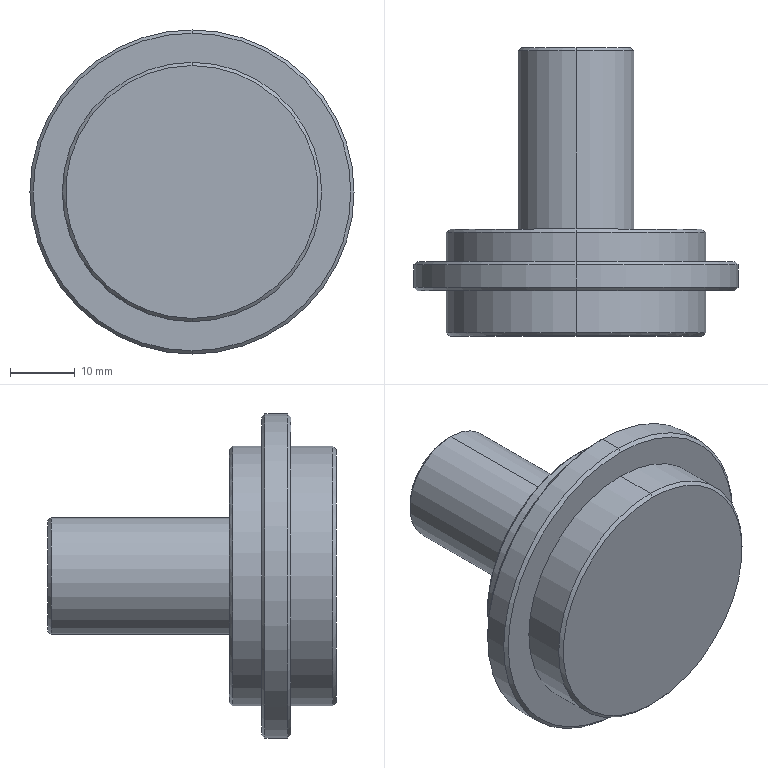Part | SolidWorks | features Chamfer 1, Revolution 1 | 1 solid | 23 faces | box 50 x 44.5 x 50 mm | volume 30963 mm3 | cone 10 | cylinder 8 | plane 5 | commonest cylinder face diameters 40 x4 18 x2 50 x2
STEP:
#1=CARTESIAN_POINT('',(249.314,-567.,8.5));
#2=VERTEX_POINT('',#1);
#3=CARTESIAN_POINT('',(249.314,-567.,-8.5));
#4=VERTEX_POINT('',#3);
#5=CARTESIAN_POINT('',(249.314,-567.,0.));
#6=DIRECTION('',(0.,1.,0.));
#7=DIRECTION('',(0.,0.,-1.));
#8=AXIS2_PLACEMENT_3D('',#5,#6,#7);
#9=CIRCLE('',#8,8.5);
#10=EDGE_CURVE('',#2,#4,#9,.T.);
#11=ORIENTED_EDGE('',*,*,#10,.F.);
#12=CARTESIAN_POINT('',(249.314,-567.5,9.));
#13=VERTEX_POINT('',#12);
#14=CARTESIAN_POINT('',(249.314,-567.,8.5));
#15=DIRECTION('',(0.,-0.7071,0.7071));
#16=VECTOR('',#15,1000.);
#17=LINE('',#14,#16);
#18=EDGE_CURVE('',#2,#13,#17,.T.);
#19=ORIENTED_EDGE('',*,*,#18,.T.);
#20=CARTESIAN_POINT('',(249.314,-567.5,-9.));
#21=VERTEX_POINT('',#20);
#22=CARTESIAN_POINT('',(249.314,-567.5,0.));
#23=DIRECTION('',(0.,-1.,0.));
#24=DIRECTION('',(0.,0.,-1.));
#25=AXIS2_PLACEMENT_3D('',#22,#23,#24);
#26=CIRCLE('',#25,9.);
#27=EDGE_CURVE('',#21,#13,#26,.T.);
#28=ORIENTED_EDGE('',*,*,#27,.F.);
#29=CARTESIAN_POINT('',(249.314,-567.,-8.5));
#30=DIRECTION('',(0.,-0.7071,-0.7071));
#31=VECTOR('',#30,1000.);
#32=LINE('',#29,#31);
#33=EDGE_CURVE('',#4,#21,#32,.T.);
#34=ORIENTED_EDGE('',*,*,#33,.F.);
#35=EDGE_LOOP('',(#11,#19,#28,#34));
#36=FACE_OUTER_BOUND('',#35,.T.);
#37=CARTESIAN_POINT('',(249.314,-567.,0.));
#38=DIRECTION('',(0.,-1.,0.));
#39=DIRECTION('',(0.,0.,-1.));
#40=AXIS2_PLACEMENT_3D('',#37,#38,#39);
#41=CONICAL_SURFACE('',#40,8.5,0.7854);
#42=ADVANCED_FACE('',(#36),#41,.T.);
#43=CARTESIAN_POINT('',(249.314,-595.,19.5));
#44=VERTEX_POINT('',#43);
#45=CARTESIAN_POINT('',(249.314,-595.,-19.5));
#46=VERTEX_POINT('',#45);
#47=CARTESIAN_POINT('',(249.314,-595.,0.));
#48=DIRECTION('',(0.,1.,0.));
#49=DIRECTION('',(0.,0.,-1.));
#50=AXIS2_PLACEMENT_3D('',#47,#48,#49);
#51=CIRCLE('',#50,19.5);
#52=EDGE_CURVE('',#44,#46,#51,.T.);
#53=ORIENTED_EDGE('',*,*,#52,.F.);
#54=CARTESIAN_POINT('',(249.314,-595.5,20.));
#55=VERTEX_POINT('',#54);
#56=CARTESIAN_POINT('',(249.314,-595.,19.5));
#57=DIRECTION('',(0.,-0.7071,0.7071));
#58=VECTOR('',#57,1000.);
#59=LINE('',#56,#58);
#60=EDGE_CURVE('',#44,#55,#59,.T.);
#61=ORIENTED_EDGE('',*,*,#60,.T.);
#62=CARTESIAN_POINT('',(249.314,-595.5,-20.));
#63=VERTEX_POINT('',#62);
#64=CARTESIAN_POINT('',(249.314,-595.5,0.));
#65=DIRECTION('',(0.,-1.,0.));
#66=DIRECTION('',(0.,0.,-1.));
#67=AXIS2_PLACEMENT_3D('',#64,#65,#66);
#68=CIRCLE('',#67,20.);
#69=EDGE_CURVE('',#63,#55,#68,.T.);
#70=ORIENTED_EDGE('',*,*,#69,.F.);
#71=CARTESIAN_POINT('',(249.314,-595.,-19.5));
#72=DIRECTION('',(0.,-0.7071,-0.7071));
#73=VECTOR('',#72,1000.);
#74=LINE('',#71,#73);
#75=EDGE_CURVE('',#46,#63,#74,.T.);
#76=ORIENTED_EDGE('',*,*,#75,.F.);
#77=EDGE_LOOP('',(#53,#61,#70,#76));
#78=FACE_OUTER_BOUND('',#77,.T.);
#79=CARTESIAN_POINT('',(249.314,-595.,0.));
#80=DIRECTION('',(0.,-1.,0.));
#81=DIRECTION('',(0.,0.,-1.));
#82=AXIS2_PLACEMENT_3D('',#79,#80,#81);
#83=CONICAL_SURFACE('',#82,19.5,0.7854);
#84=ADVANCED_FACE('',(#78),#83,.T.);
#85=CARTESIAN_POINT('',(249.314,-600.,24.5));
#86=VERTEX_POINT('',#85);
#87=CARTESIAN_POINT('',(249.314,-600.,-24.5));
#88=VERTEX_POINT('',#87);
#89=CARTESIAN_POINT('',(249.314,-600.,0.));
#90=DIRECTION('',(0.,1.,0.));
#91=DIRECTION('',(0.,0.,-1.));
#92=AXIS2_PLACEMENT_3D('',#89,#90,#91);
#93=CIRCLE('',#92,24.5);
#94=EDGE_CURVE('',#86,#88,#93,.T.);
#95=ORIENTED_EDGE('',*,*,#94,.F.);
#96=CARTESIAN_POINT('',(249.314,-600.5,25.));
#97=VERTEX_POINT('',#96);
#98=CARTESIAN_POINT('',(249.314,-600.,24.5));
#99=DIRECTION('',(0.,-0.7071,0.7071));
#100=VECTOR('',#99,1000.);
#101=LINE('',#98,#100);
#102=EDGE_CURVE('',#86,#97,#101,.T.);
#103=ORIENTED_EDGE('',*,*,#102,.T.);
#104=CARTESIAN_POINT('',(249.314,-600.5,-25.));
#105=VERTEX_POINT('',#104);
#106=CARTESIAN_POINT('',(249.314,-600.5,0.));
#107=DIRECTION('',(0.,-1.,0.));
#108=DIRECTION('',(0.,0.,-1.));
#109=AXIS2_PLACEMENT_3D('',#106,#107,#108);
#110=CIRCLE('',#109,25.);
#111=EDGE_CURVE('',#105,#97,#110,.T.);
#112=ORIENTED_EDGE('',*,*,#111,.F.);
#113=CARTESIAN_POINT('',(249.314,-600.,-24.5));
#114=DIRECTION('',(0.,-0.7071,-0.7071));
#115=VECTOR('',#114,1000.);
#116=LINE('',#113,#115);
#117=EDGE_CURVE('',#88,#105,#116,.T.);
#118=ORIENTED_EDGE('',*,*,#117,.F.);
#119=EDGE_LOOP('',(#95,#103,#112,#118));
#120=FACE_OUTER_BOUND('',#119,.T.);
#121=CARTESIAN_POINT('',(249.314,-600.,0.));
#122=DIRECTION('',(0.,-1.,0.));
#123=DIRECTION('',(0.,0.,-1.));
#124=AXIS2_PLACEMENT_3D('',#121,#122,#123);
#125=CONICAL_SURFACE('',#124,24.5,0.7854);
#126=ADVANCED_FACE('',(#120),#125,.T.);
#127=CARTESIAN_POINT('',(249.314,-604.5,-24.5));
#128=VERTEX_POINT('',#127);
#129=CARTESIAN_POINT('',(249.314,-604.5,24.5));
#130=VERTEX_POINT('',#129);
#131=CARTESIAN_POINT('',(249.314,-604.5,0.));
#132=DIRECTION('',(0.,-1.,0.));
#133=DIRECTION('',(0.,0.,1.));
#134=AXIS2_PLACEMENT_3D('',#131,#132,#133);
#135=CIRCLE('',#134,24.5);
#136=EDGE_CURVE('',#128,#130,#135,.T.);
#137=ORIENTED_EDGE('',*,*,#136,.F.);
#138=CARTESIAN_POINT('',(249.314,-604.,-25.));
#139=VERTEX_POINT('',#138);
#140=CARTESIAN_POINT('',(249.314,-604.,-25.));
#141=DIRECTION('',(0.,0.7071,-0.7071));
#142=VECTOR('',#141,1000.);
#143=LINE('',#140,#142);
#144=EDGE_CURVE('',#128,#139,#143,.T.);
#145=ORIENTED_EDGE('',*,*,#144,.T.);
#146=CARTESIAN_POINT('',(249.314,-604.,25.));
#147=VERTEX_POINT('',#146);
#148=CARTESIAN_POINT('',(249.314,-604.,0.));
#149=DIRECTION('',(0.,1.,0.));
#150=DIRECTION('',(0.,0.,1.));
#151=AXIS2_PLACEMENT_3D('',#148,#149,#150);
#152=CIRCLE('',#151,25.);
#153=EDGE_CURVE('',#147,#139,#152,.T.);
#154=ORIENTED_EDGE('',*,*,#153,.F.);
#155=CARTESIAN_POINT('',(249.314,-604.,25.));
#156=DIRECTION('',(0.,0.7071,0.7071));
#157=VECTOR('',#156,1000.);
#158=LINE('',#155,#157);
#159=EDGE_CURVE('',#130,#147,#158,.T.);
#160=ORIENTED_EDGE('',*,*,#159,.F.);
#161=EDGE_LOOP('',(#137,#145,#154,#160));
#162=FACE_OUTER_BOUND('',#161,.T.);
#163=CARTESIAN_POINT('',(249.314,-604.,0.));
#164=DIRECTION('',(0.,1.,0.));
#165=DIRECTION('',(0.,0.,1.));
#166=AXIS2_PLACEMENT_3D('',#163,#164,#165);
#167=CONICAL_SURFACE('',#166,25.,0.7854);
#168=ADVANCED_FACE('',(#162),#167,.T.);
#169=CARTESIAN_POINT('',(249.314,-611.5,-19.5));
#170=VERTEX_POINT('',#169);
#171=CARTESIAN_POINT('',(249.314,-611.5,19.5));
#172=VERTEX_POINT('',#171);
#173=CARTESIAN_POINT('',(249.314,-611.5,0.));
#174=DIRECTION('',(0.,-1.,0.));
#175=DIRECTION('',(0.,0.,1.));
#176=AXIS2_PLACEMENT_3D('',#173,#174,#175);
#177=CIRCLE('',#176,19.5);
#178=EDGE_CURVE('',#170,#172,#177,.T.);
#179=ORIENTED_EDGE('',*,*,#178,.F.);
#180=CARTESIAN_POINT('',(249.314,-611.,-20.));
#181=VERTEX_POINT('',#180);
#182=CARTESIAN_POINT('',(249.314,-611.,-20.));
#183=DIRECTION('',(0.,0.7071,-0.7071));
#184=VECTOR('',#183,1000.);
#185=LINE('',#182,#184);
#186=EDGE_CURVE('',#170,#181,#185,.T.);
#187=ORIENTED_EDGE('',*,*,#186,.T.);
#188=CARTESIAN_POINT('',(249.314,-611.,20.));
#189=VERTEX_POINT('',#188);
#190=CARTESIAN_POINT('',(249.314,-611.,0.));
#191=DIRECTION('',(0.,1.,0.));
#192=DIRECTION('',(0.,0.,1.));
#193=AXIS2_PLACEMENT_3D('',#190,#191,#192);
#194=CIRCLE('',#193,20.);
#195=EDGE_CURVE('',#189,#181,#194,.T.);
#196=ORIENTED_EDGE('',*,*,#195,.F.);
#197=CARTESIAN_POINT('',(249.314,-611.,20.));
#198=DIRECTION('',(0.,0.7071,0.7071));
#199=VECTOR('',#198,1000.);
#200=LINE('',#197,#199);
#201=EDGE_CURVE('',#172,#189,#200,.T.);
#202=ORIENTED_EDGE('',*,*,#201,.F.);
#203=EDGE_LOOP('',(#179,#187,#196,#202));
#204=FACE_OUTER_BOUND('',#203,.T.);
#205=CARTESIAN_POINT('',(249.314,-611.,0.));
#206=DIRECTION('',(0.,1.,0.));
#207=DIRECTION('',(0.,0.,1.));
#208=AXIS2_PLACEMENT_3D('',#205,#206,#207);
#209=CONICAL_SURFACE('',#208,20.,0.7854);
#210=ADVANCED_FACE('',(#204),#209,.T.);
#211=CARTESIAN_POINT('',(249.314,-595.,9.));
#212=VERTEX_POINT('',#211);
#213=CARTESIAN_POINT('',(249.314,-595.,-9.));
#214=VERTEX_POINT('',#213);
#215=CARTESIAN_POINT('',(249.314,-595.,0.));
#216=DIRECTION('',(0.,1.,0.));
#217=DIRECTION('',(0.,0.,1.));
#218=AXIS2_PLACEMENT_3D('',#215,#216,#217);
#219=CIRCLE('',#218,9.);
#220=EDGE_CURVE('',#212,#214,#219,.T.);
#221=ORIENTED_EDGE('',*,*,#220,.T.);
#222=CARTESIAN_POINT('',(249.314,-567.,-9.));
#223=DIRECTION('',(0.,1.,0.));
#224=VECTOR('',#223,1000.);
#225=LINE('',#222,#224);
#226=EDGE_CURVE('',#214,#21,#225,.T.);
#227=ORIENTED_EDGE('',*,*,#226,.T.);
#228=ORIENTED_EDGE('',*,*,#27,.T.);
#229=CARTESIAN_POINT('',(249.314,-567.,9.));
#230=DIRECTION('',(0.,1.,0.));
#231=VECTOR('',#230,1000.);
#232=LINE('',#229,#231);
#233=EDGE_CURVE('',#212,#13,#232,.T.);
#234=ORIENTED_EDGE('',*,*,#233,.F.);
#235=EDGE_LOOP('',(#221,#227,#228,#234));
#236=FACE_OUTER_BOUND('',#235,.T.);
#237=CARTESIAN_POINT('',(249.314,-567.,0.));
#238=DIRECTION('',(0.,1.,0.));
#239=DIRECTION('',(0.,0.,1.));
#240=AXIS2_PLACEMENT_3D('',#237,#238,#239);
#241=CYLINDRICAL_SURFACE('',#240,9.);
#242=ADVANCED_FACE('',(#236),#241,.T.);
#243=CARTESIAN_POINT('',(249.314,-600.,20.));
#244=VERTEX_POINT('',#243);
#245=CARTESIAN_POINT('',(249.314,-600.,-20.));
#246=VERTEX_POINT('',#245);
#247=CARTESIAN_POINT('',(249.314,-600.,0.));
#248=DIRECTION('',(0.,1.,0.));
#249=DIRECTION('',(0.,0.,1.));
#250=AXIS2_PLACEMENT_3D('',#247,#248,#249);
#251=CIRCLE('',#250,20.);
#252=EDGE_CURVE('',#244,#246,#251,.T.);
#253=ORIENTED_EDGE('',*,*,#252,.T.);
#254=CARTESIAN_POINT('',(249.314,-567.,-20.));
#255=DIRECTION('',(0.,1.,0.));
#256=VECTOR('',#255,1000.);
#257=LINE('',#254,#256);
#258=EDGE_CURVE('',#246,#63,#257,.T.);
#259=ORIENTED_EDGE('',*,*,#258,.T.);
#260=ORIENTED_EDGE('',*,*,#69,.T.);
#261=CARTESIAN_POINT('',(249.314,-567.,20.));
#262=DIRECTION('',(0.,1.,0.));
#263=VECTOR('',#262,1000.);
#264=LINE('',#261,#263);
#265=EDGE_CURVE('',#244,#55,#264,.T.);
#266=ORIENTED_EDGE('',*,*,#265,.F.);
#267=EDGE_LOOP('',(#253,#259,#260,#266));
#268=FACE_OUTER_BOUND('',#267,.T.);
#269=CARTESIAN_POINT('',(249.314,-567.,0.));
#270=DIRECTION('',(0.,1.,0.));
#271=DIRECTION('',(0.,0.,1.));
#272=AXIS2_PLACEMENT_3D('',#269,#270,#271);
#273=CYLINDRICAL_SURFACE('',#272,20.);
#274=ADVANCED_FACE('',(#268),#273,.T.);
#275=ORIENTED_EDGE('',*,*,#153,.T.);
#276=CARTESIAN_POINT('',(249.314,-567.,-25.));
#277=DIRECTION('',(0.,1.,0.));
#278=VECTOR('',#277,1000.);
#279=LINE('',#276,#278);
#280=EDGE_CURVE('',#139,#105,#279,.T.);
#281=ORIENTED_EDGE('',*,*,#280,.T.);
#282=ORIENTED_EDGE('',*,*,#111,.T.);
#283=CARTESIAN_POINT('',(249.314,-567.,25.));
#284=DIRECTION('',(0.,1.,0.));
#285=VECTOR('',#284,1000.);
#286=LINE('',#283,#285);
#287=EDGE_CURVE('',#147,#97,#286,.T.);
#288=ORIENTED_EDGE('',*,*,#287,.F.);
#289=EDGE_LOOP('',(#275,#281,#282,#288));
#290=FACE_OUTER_BOUND('',#289,.T.);
#291=CARTESIAN_POINT('',(249.314,-567.,0.));
#292=DIRECTION('',(0.,1.,0.));
#293=DIRECTION('',(0.,0.,1.));
#294=AXIS2_PLACEMENT_3D('',#291,#292,#293);
#295=CYLINDRICAL_SURFACE('',#294,25.);
#296=ADVANCED_FACE('',(#290),#295,.T.);
#297=ORIENTED_EDGE('',*,*,#195,.T.);
#298=CARTESIAN_POINT('',(249.314,-604.5,-20.));
#299=VERTEX_POINT('',#298);
#300=CARTESIAN_POINT('',(249.314,-567.,-20.));
#301=DIRECTION('',(0.,1.,0.));
#302=VECTOR('',#301,1000.);
#303=LINE('',#300,#302);
#304=EDGE_CURVE('',#181,#299,#303,.T.);
#305=ORIENTED_EDGE('',*,*,#304,.T.);
#306=CARTESIAN_POINT('',(249.314,-604.5,20.));
#307=VERTEX_POINT('',#306);
#308=CARTESIAN_POINT('',(249.314,-604.5,0.));
#309=DIRECTION('',(0.,1.,0.));
#310=DIRECTION('',(0.,0.,1.));
#311=AXIS2_PLACEMENT_3D('',#308,#309,#310);
#312=CIRCLE('',#311,20.);
#313=EDGE_CURVE('',#307,#299,#312,.T.);
#314=ORIENTED_EDGE('',*,*,#313,.F.);
#315=CARTESIAN_POINT('',(249.314,-567.,20.));
#316=DIRECTION('',(0.,1.,0.));
#317=VECTOR('',#316,1000.);
#318=LINE('',#315,#317);
#319=EDGE_CURVE('',#189,#307,#318,.T.);
#320=ORIENTED_EDGE('',*,*,#319,.F.);
#321=EDGE_LOOP('',(#297,#305,#314,#320));
#322=FACE_OUTER_BOUND('',#321,.T.);
#323=CARTESIAN_POINT('',(249.314,-567.,0.));
#324=DIRECTION('',(0.,1.,0.));
#325=DIRECTION('',(0.,0.,1.));
#326=AXIS2_PLACEMENT_3D('',#323,#324,#325);
#327=CYLINDRICAL_SURFACE('',#326,20.);
#328=ADVANCED_FACE('',(#322),#327,.T.);
#329=CARTESIAN_POINT('',(249.314,-567.,0.));
#330=DIRECTION('',(0.,1.,0.));
#331=DIRECTION('',(0.,0.,-1.));
#332=AXIS2_PLACEMENT_3D('',#329,#330,#331);
#333=CIRCLE('',#332,8.5);
#334=EDGE_CURVE('',#4,#2,#333,.T.);
#335=ORIENTED_EDGE('',*,*,#334,.T.);
#336=ORIENTED_EDGE('',*,*,#10,.T.);
#337=EDGE_LOOP('',(#335,#336));
#338=FACE_OUTER_BOUND('',#337,.T.);
#339=CARTESIAN_POINT('',(258.314,-567.,0.));
#340=DIRECTION('',(0.,-1.,0.));
#341=DIRECTION('',(0.,0.,-1.));
#342=AXIS2_PLACEMENT_3D('',#339,#340,#341);
#343=PLANE('',#342);
#344=ADVANCED_FACE('',(#338),#343,.F.);
#345=CARTESIAN_POINT('',(249.314,-611.5,0.));
#346=DIRECTION('',(0.,-1.,0.));
#347=DIRECTION('',(0.,0.,1.));
#348=AXIS2_PLACEMENT_3D('',#345,#346,#347);
#349=CIRCLE('',#348,19.5);
#350=EDGE_CURVE('',#172,#170,#349,.T.);
#351=ORIENTED_EDGE('',*,*,#350,.T.);
#352=ORIENTED_EDGE('',*,*,#178,.T.);
#353=EDGE_LOOP('',(#351,#352));
#354=FACE_OUTER_BOUND('',#353,.T.);
#355=CARTESIAN_POINT('',(269.314,-611.5,0.));
#356=DIRECTION('',(0.,1.,0.));
#357=DIRECTION('',(0.,0.,1.));
#358=AXIS2_PLACEMENT_3D('',#355,#356,#357);
#359=PLANE('',#358);
#360=ADVANCED_FACE('',(#354),#359,.F.);
#361=ORIENTED_EDGE('',*,*,#304,.F.);
#362=CARTESIAN_POINT('',(249.314,-611.,0.));
#363=DIRECTION('',(0.,1.,0.));
#364=DIRECTION('',(0.,0.,1.));
#365=AXIS2_PLACEMENT_3D('',#362,#363,#364);
#366=CIRCLE('',#365,20.);
#367=EDGE_CURVE('',#181,#189,#366,.T.);
#368=ORIENTED_EDGE('',*,*,#367,.T.);
#369=ORIENTED_EDGE('',*,*,#319,.T.);
#370=CARTESIAN_POINT('',(249.314,-604.5,0.));
#371=DIRECTION('',(0.,1.,0.));
#372=DIRECTION('',(0.,0.,1.));
#373=AXIS2_PLACEMENT_3D('',#370,#371,#372);
#374=CIRCLE('',#373,20.);
#375=EDGE_CURVE('',#299,#307,#374,.T.);
#376=ORIENTED_EDGE('',*,*,#375,.F.);
#377=EDGE_LOOP('',(#361,#368,#369,#376));
#378=FACE_OUTER_BOUND('',#377,.T.);
#379=CARTESIAN_POINT('',(249.314,-567.,0.));
#380=DIRECTION('',(0.,1.,0.));
#381=DIRECTION('',(0.,0.,1.));
#382=AXIS2_PLACEMENT_3D('',#379,#380,#381);
#383=CYLINDRICAL_SURFACE('',#382,20.);
#384=ADVANCED_FACE('',(#378),#383,.T.);
#385=CARTESIAN_POINT('',(249.314,-604.5,0.));
#386=DIRECTION('',(0.,-1.,0.));
#387=DIRECTION('',(0.,0.,1.));
#388=AXIS2_PLACEMENT_3D('',#385,#386,#387);
#389=CIRCLE('',#388,24.5);
#390=EDGE_CURVE('',#130,#128,#389,.T.);
#391=ORIENTED_EDGE('',*,*,#390,.T.);
#392=ORIENTED_EDGE('',*,*,#136,.T.);
#393=EDGE_LOOP('',(#391,#392));
#394=FACE_OUTER_BOUND('',#393,.T.);
#395=ORIENTED_EDGE('',*,*,#313,.T.);
#396=ORIENTED_EDGE('',*,*,#375,.T.);
#397=EDGE_LOOP('',(#395,#396));
#398=FACE_BOUND('',#397,.T.);
#399=CARTESIAN_POINT('',(274.314,-604.5,0.));
#400=DIRECTION('',(0.,1.,0.));
#401=DIRECTION('',(0.,0.,1.));
#402=AXIS2_PLACEMENT_3D('',#399,#400,#401);
#403=PLANE('',#402);
#404=ADVANCED_FACE('',(#394,#398),#403,.F.);
#405=ORIENTED_EDGE('',*,*,#280,.F.);
#406=CARTESIAN_POINT('',(249.314,-604.,0.));
#407=DIRECTION('',(0.,1.,0.));
#408=DIRECTION('',(0.,0.,1.));
#409=AXIS2_PLACEMENT_3D('',#406,#407,#408);
#410=CIRCLE('',#409,25.);
#411=EDGE_CURVE('',#139,#147,#410,.T.);
#412=ORIENTED_EDGE('',*,*,#411,.T.);
#413=ORIENTED_EDGE('',*,*,#287,.T.);
#414=CARTESIAN_POINT('',(249.314,-600.5,0.));
#415=DIRECTION('',(0.,-1.,0.));
#416=DIRECTION('',(0.,0.,-1.));
#417=AXIS2_PLACEMENT_3D('',#414,#415,#416);
#418=CIRCLE('',#417,25.);
#419=EDGE_CURVE('',#97,#105,#418,.T.);
#420=ORIENTED_EDGE('',*,*,#419,.T.);
#421=EDGE_LOOP('',(#405,#412,#413,#420));
#422=FACE_OUTER_BOUND('',#421,.T.);
#423=CARTESIAN_POINT('',(249.314,-567.,0.));
#424=DIRECTION('',(0.,1.,0.));
#425=DIRECTION('',(0.,0.,1.));
#426=AXIS2_PLACEMENT_3D('',#423,#424,#425);
#427=CYLINDRICAL_SURFACE('',#426,25.);
#428=ADVANCED_FACE('',(#422),#427,.T.);
#429=CARTESIAN_POINT('',(249.314,-600.,0.));
#430=DIRECTION('',(0.,1.,0.));
#431=DIRECTION('',(0.,0.,-1.));
#432=AXIS2_PLACEMENT_3D('',#429,#430,#431);
#433=CIRCLE('',#432,24.5);
#434=EDGE_CURVE('',#88,#86,#433,.T.);
#435=ORIENTED_EDGE('',*,*,#434,.T.);
#436=ORIENTED_EDGE('',*,*,#94,.T.);
#437=EDGE_LOOP('',(#435,#436));
#438=FACE_OUTER_BOUND('',#437,.T.);
#439=ORIENTED_EDGE('',*,*,#252,.F.);
#440=CARTESIAN_POINT('',(249.314,-600.,0.));
#441=DIRECTION('',(0.,1.,0.));
#442=DIRECTION('',(0.,0.,1.));
#443=AXIS2_PLACEMENT_3D('',#440,#441,#442);
#444=CIRCLE('',#443,20.);
#445=EDGE_CURVE('',#246,#244,#444,.T.);
#446=ORIENTED_EDGE('',*,*,#445,.F.);
#447=EDGE_LOOP('',(#439,#446));
#448=FACE_BOUND('',#447,.T.);
#449=CARTESIAN_POINT('',(269.314,-600.,0.));
#450=DIRECTION('',(0.,-1.,0.));
#451=DIRECTION('',(0.,0.,-1.));
#452=AXIS2_PLACEMENT_3D('',#449,#450,#451);
#453=PLANE('',#452);
#454=ADVANCED_FACE('',(#438,#448),#453,.F.);
#455=ORIENTED_EDGE('',*,*,#258,.F.);
#456=ORIENTED_EDGE('',*,*,#445,.T.);
#457=ORIENTED_EDGE('',*,*,#265,.T.);
#458=CARTESIAN_POINT('',(249.314,-595.5,0.));
#459=DIRECTION('',(0.,-1.,0.));
#460=DIRECTION('',(0.,0.,-1.));
#461=AXIS2_PLACEMENT_3D('',#458,#459,#460);
#462=CIRCLE('',#461,20.);
#463=EDGE_CURVE('',#55,#63,#462,.T.);
#464=ORIENTED_EDGE('',*,*,#463,.T.);
#465=EDGE_LOOP('',(#455,#456,#457,#464));
#466=FACE_OUTER_BOUND('',#465,.T.);
#467=CARTESIAN_POINT('',(249.314,-567.,0.));
#468=DIRECTION('',(0.,1.,0.));
#469=DIRECTION('',(0.,0.,1.));
#470=AXIS2_PLACEMENT_3D('',#467,#468,#469);
#471=CYLINDRICAL_SURFACE('',#470,20.);
#472=ADVANCED_FACE('',(#466),#471,.T.);
#473=CARTESIAN_POINT('',(249.314,-595.,0.));
#474=DIRECTION('',(0.,1.,0.));
#475=DIRECTION('',(0.,0.,-1.));
#476=AXIS2_PLACEMENT_3D('',#473,#474,#475);
#477=CIRCLE('',#476,19.5);
#478=EDGE_CURVE('',#46,#44,#477,.T.);
#479=ORIENTED_EDGE('',*,*,#478,.T.);
#480=ORIENTED_EDGE('',*,*,#52,.T.);
#481=EDGE_LOOP('',(#479,#480));
#482=FACE_OUTER_BOUND('',#481,.T.);
#483=ORIENTED_EDGE('',*,*,#220,.F.);
#484=CARTESIAN_POINT('',(249.314,-595.,0.));
#485=DIRECTION('',(0.,1.,0.));
#486=DIRECTION('',(0.,0.,1.));
#487=AXIS2_PLACEMENT_3D('',#484,#485,#486);
#488=CIRCLE('',#487,9.);
#489=EDGE_CURVE('',#214,#212,#488,.T.);
#490=ORIENTED_EDGE('',*,*,#489,.F.);
#491=EDGE_LOOP('',(#483,#490));
#492=FACE_BOUND('',#491,.T.);
#493=CARTESIAN_POINT('',(258.314,-595.,0.));
#494=DIRECTION('',(0.,-1.,0.));
#495=DIRECTION('',(0.,0.,-1.));
#496=AXIS2_PLACEMENT_3D('',#493,#494,#495);
#497=PLANE('',#496);
#498=ADVANCED_FACE('',(#482,#492),#497,.F.);
#499=ORIENTED_EDGE('',*,*,#226,.F.);
#500=ORIENTED_EDGE('',*,*,#489,.T.);
#501=ORIENTED_EDGE('',*,*,#233,.T.);
#502=CARTESIAN_POINT('',(249.314,-567.5,0.));
#503=DIRECTION('',(0.,-1.,0.));
#504=DIRECTION('',(0.,0.,-1.));
#505=AXIS2_PLACEMENT_3D('',#502,#503,#504);
#506=CIRCLE('',#505,9.);
#507=EDGE_CURVE('',#13,#21,#506,.T.);
#508=ORIENTED_EDGE('',*,*,#507,.T.);
#509=EDGE_LOOP('',(#499,#500,#501,#508));
#510=FACE_OUTER_BOUND('',#509,.T.);
#511=CARTESIAN_POINT('',(249.314,-567.,0.));
#512=DIRECTION('',(0.,1.,0.));
#513=DIRECTION('',(0.,0.,1.));
#514=AXIS2_PLACEMENT_3D('',#511,#512,#513);
#515=CYLINDRICAL_SURFACE('',#514,9.);
#516=ADVANCED_FACE('',(#510),#515,.T.);
#517=ORIENTED_EDGE('',*,*,#186,.F.);
#518=ORIENTED_EDGE('',*,*,#350,.F.);
#519=ORIENTED_EDGE('',*,*,#201,.T.);
#520=ORIENTED_EDGE('',*,*,#367,.F.);
#521=EDGE_LOOP('',(#517,#518,#519,#520));
#522=FACE_OUTER_BOUND('',#521,.T.);
#523=CARTESIAN_POINT('',(249.314,-611.,0.));
#524=DIRECTION('',(0.,1.,0.));
#525=DIRECTION('',(0.,0.,1.));
#526=AXIS2_PLACEMENT_3D('',#523,#524,#525);
#527=CONICAL_SURFACE('',#526,20.,0.7854);
#528=ADVANCED_FACE('',(#522),#527,.T.);
#529=ORIENTED_EDGE('',*,*,#144,.F.);
#530=ORIENTED_EDGE('',*,*,#390,.F.);
#531=ORIENTED_EDGE('',*,*,#159,.T.);
#532=ORIENTED_EDGE('',*,*,#411,.F.);
#533=EDGE_LOOP('',(#529,#530,#531,#532));
#534=FACE_OUTER_BOUND('',#533,.T.);
#535=CARTESIAN_POINT('',(249.314,-604.,0.));
#536=DIRECTION('',(0.,1.,0.));
#537=DIRECTION('',(0.,0.,1.));
#538=AXIS2_PLACEMENT_3D('',#535,#536,#537);
#539=CONICAL_SURFACE('',#538,25.,0.7854);
#540=ADVANCED_FACE('',(#534),#539,.T.);
#541=ORIENTED_EDGE('',*,*,#102,.F.);
#542=ORIENTED_EDGE('',*,*,#434,.F.);
#543=ORIENTED_EDGE('',*,*,#117,.T.);
#544=ORIENTED_EDGE('',*,*,#419,.F.);
#545=EDGE_LOOP('',(#541,#542,#543,#544));
#546=FACE_OUTER_BOUND('',#545,.T.);
#547=CARTESIAN_POINT('',(249.314,-600.,0.));
#548=DIRECTION('',(0.,-1.,0.));
#549=DIRECTION('',(0.,0.,-1.));
#550=AXIS2_PLACEMENT_3D('',#547,#548,#549);
#551=CONICAL_SURFACE('',#550,24.5,0.7854);
#552=ADVANCED_FACE('',(#546),#551,.T.);
#553=ORIENTED_EDGE('',*,*,#60,.F.);
#554=ORIENTED_EDGE('',*,*,#478,.F.);
#555=ORIENTED_EDGE('',*,*,#75,.T.);
#556=ORIENTED_EDGE('',*,*,#463,.F.);
#557=EDGE_LOOP('',(#553,#554,#555,#556));
#558=FACE_OUTER_BOUND('',#557,.T.);
#559=CARTESIAN_POINT('',(249.314,-595.,0.));
#560=DIRECTION('',(0.,-1.,0.));
#561=DIRECTION('',(0.,0.,-1.));
#562=AXIS2_PLACEMENT_3D('',#559,#560,#561);
#563=CONICAL_SURFACE('',#562,19.5,0.7854);
#564=ADVANCED_FACE('',(#558),#563,.T.);
#565=ORIENTED_EDGE('',*,*,#18,.F.);
#566=ORIENTED_EDGE('',*,*,#334,.F.);
#567=ORIENTED_EDGE('',*,*,#33,.T.);
#568=ORIENTED_EDGE('',*,*,#507,.F.);
#569=EDGE_LOOP('',(#565,#566,#567,#568));
#570=FACE_OUTER_BOUND('',#569,.T.);
#571=CARTESIAN_POINT('',(249.314,-567.,0.));
#572=DIRECTION('',(0.,-1.,0.));
#573=DIRECTION('',(0.,0.,-1.));
#574=AXIS2_PLACEMENT_3D('',#571,#572,#573);
#575=CONICAL_SURFACE('',#574,8.5,0.7854);
#576=ADVANCED_FACE('',(#570),#575,.T.);
#577=CLOSED_SHELL('',(#42,#84,#126,#168,#210,#242,#274,#296,#328,#344,#360,#384,#404,#428,#454,#472,#498,#516,#528,#540,#552,#564,#576));
#578=MANIFOLD_SOLID_BREP('',#577);
#579=CARTESIAN_POINT('',(0.,0.,0.));
#580=DIRECTION('',(0.,0.,1.));
#581=DIRECTION('',(1.,0.,0.));
#582=AXIS2_PLACEMENT_3D('',#579,#580,#581);
#583=(LENGTH_UNIT()NAMED_UNIT(*)SI_UNIT(.MILLI.,.METRE.));
#584=UNCERTAINTY_MEASURE_WITH_UNIT(LENGTH_MEASURE(0.00001),#583,'','');
#585=(NAMED_UNIT(*)PLANE_ANGLE_UNIT()SI_UNIT($,.RADIAN.));
#586=(NAMED_UNIT(*)SI_UNIT($,.STERADIAN.)SOLID_ANGLE_UNIT());
#587=(GEOMETRIC_REPRESENTATION_CONTEXT(3)GLOBAL_UNCERTAINTY_ASSIGNED_CONTEXT((#584))GLOBAL_UNIT_ASSIGNED_CONTEXT((#583,#585,#586))REPRESENTATION_CONTEXT('',''));
#588=ADVANCED_BREP_SHAPE_REPRESENTATION('',(#578,#582),#587);